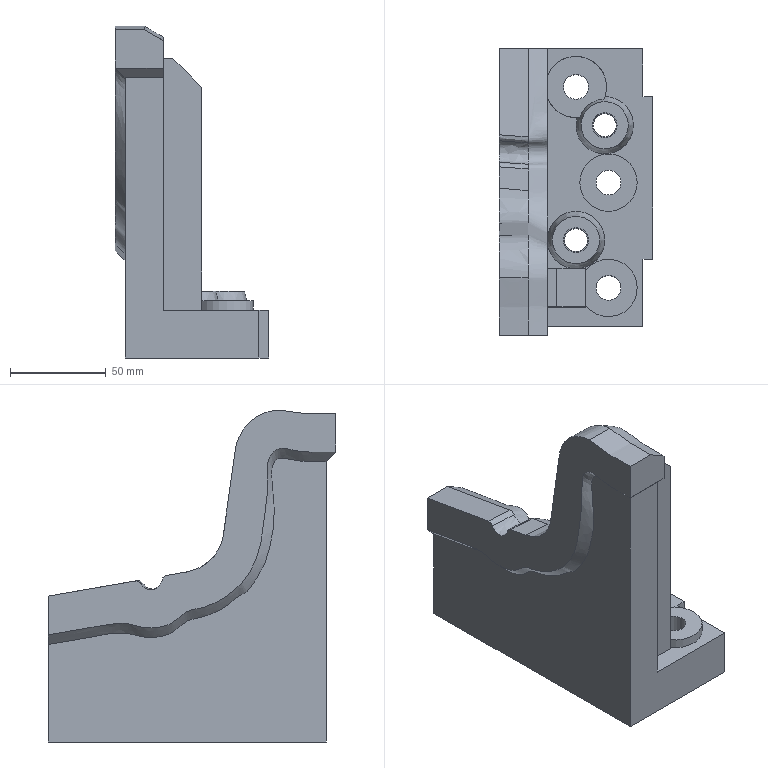Part | NX | features solid 2 | 1 solid | 50 faces | box 80 x 150.066 x 173.499 mm | volume 593373 mm3 | plane 23 | spline 14 | cylinder 11 | cone 2 | commonest cylinder face diameters 13 x5 12 x2 30 x2 32 x2